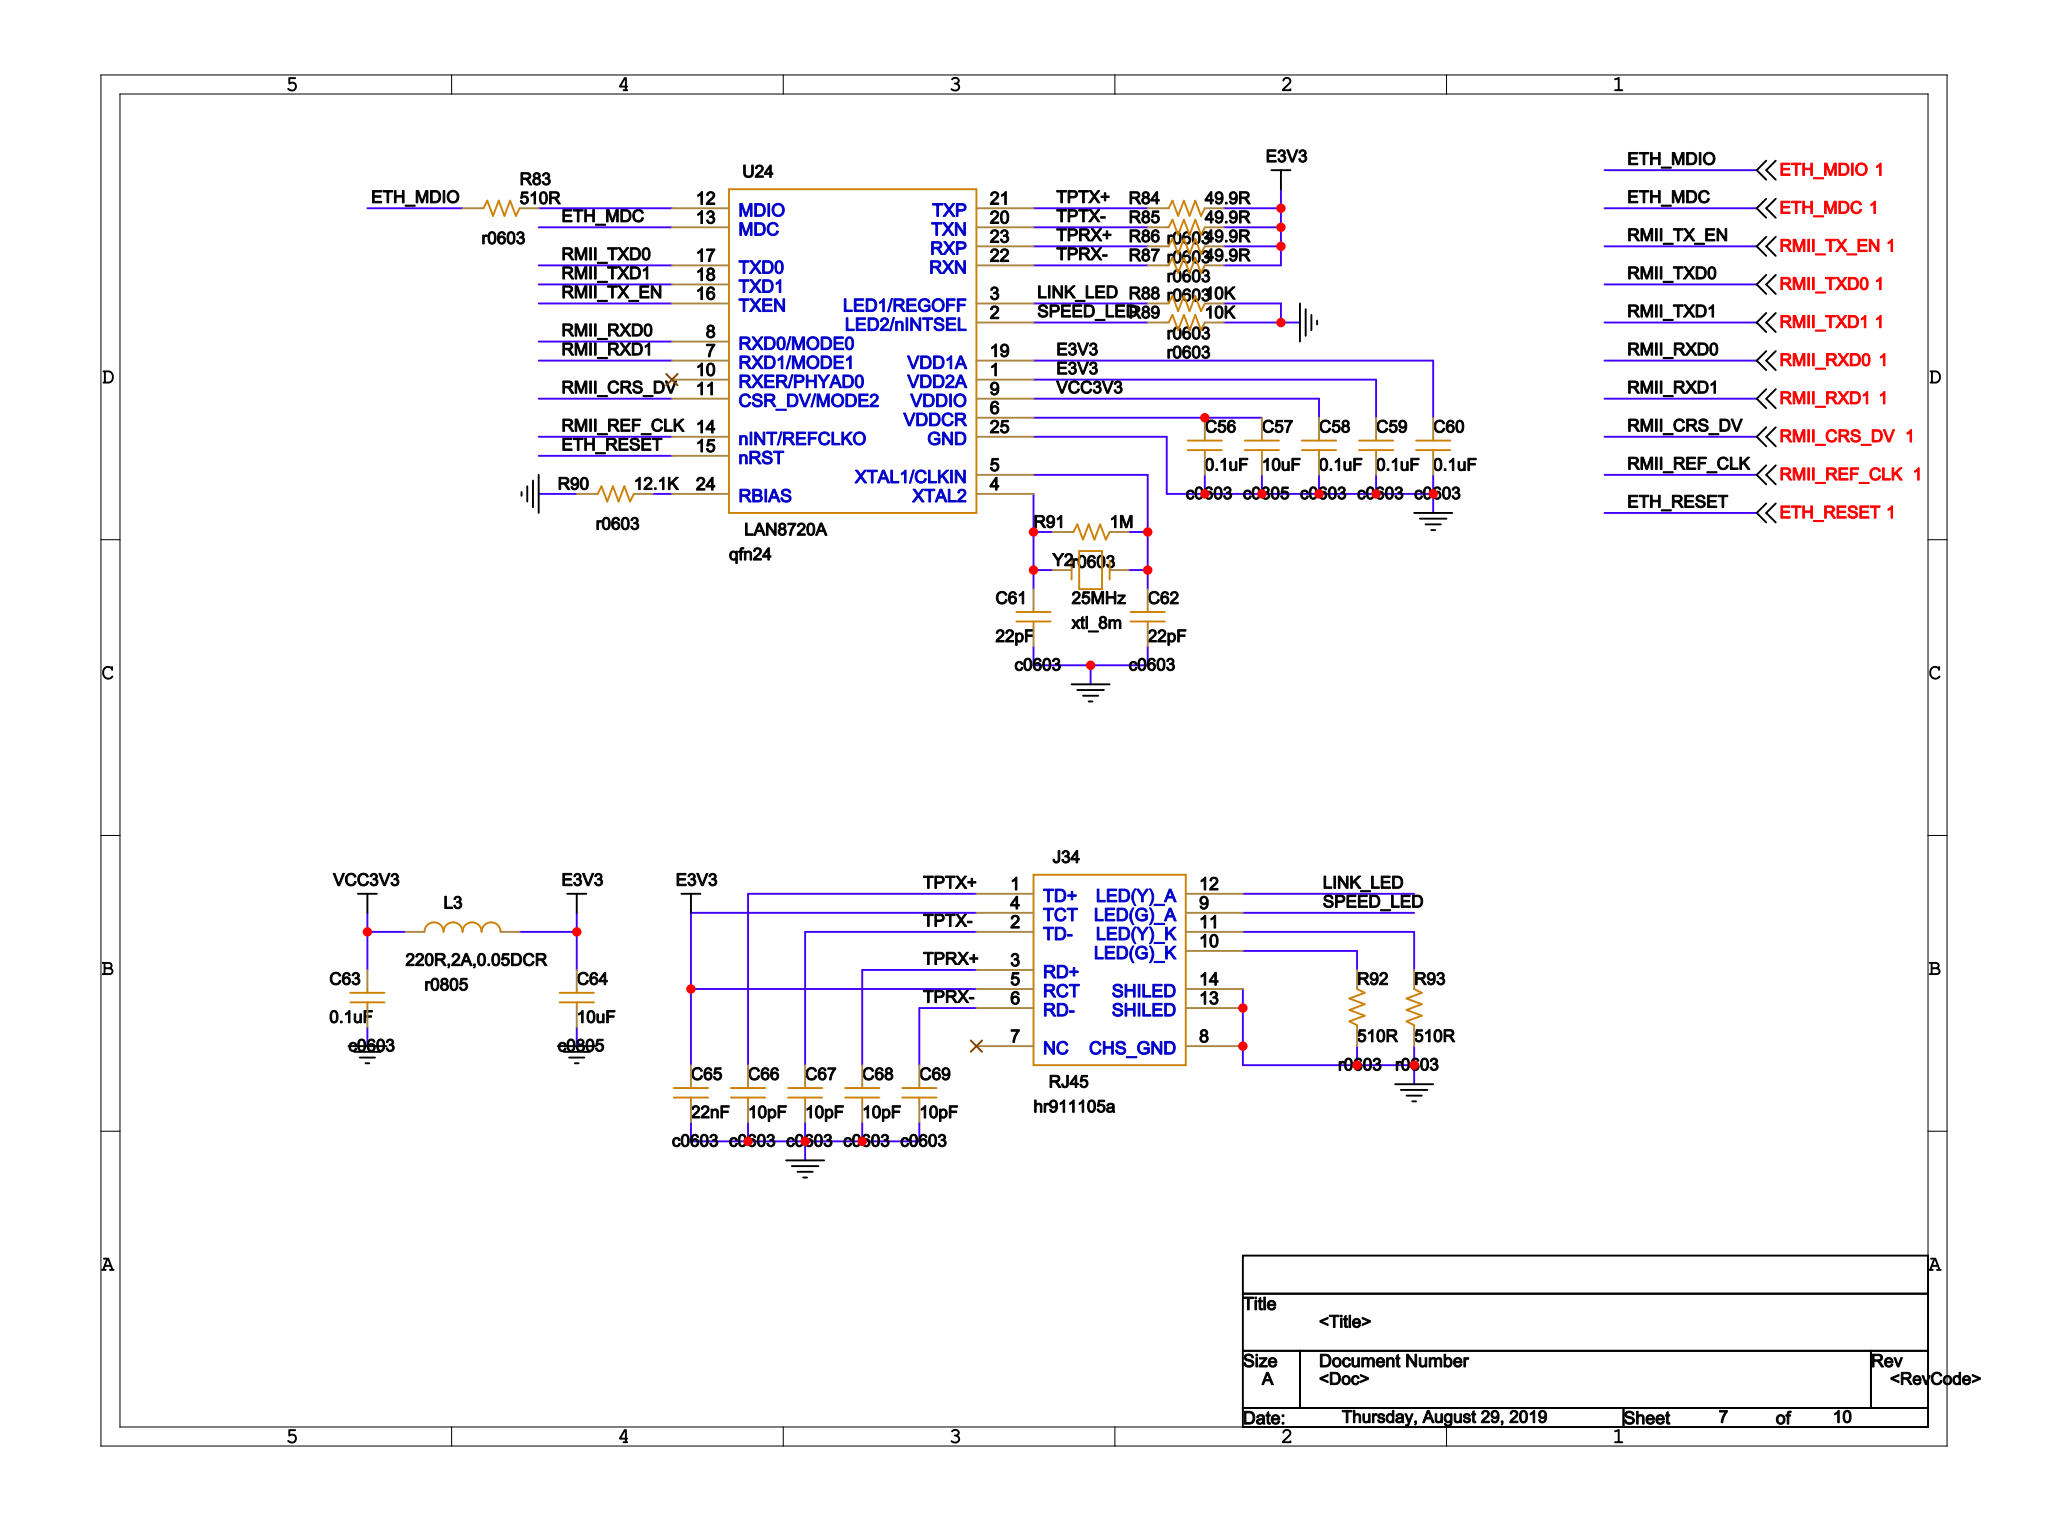Circuit board | Cadence Allegro | 380 parts | 375 nets | one sheet of the schematic
Parts on this sheet (reference | value | footprint):
C56 | 0.1uF | C0603
C57 | 10uF | C0805
C58 | 0.1uF | C0603
C59 | 0.1uF | C0603
C60 | 0.1uF | C0603
C61 | 22pF | C0603
C62 | 22pF | C0603
C63 | 0.1uF | C0603
C64 | 10uF | C0805
C65 | 22nF | C0603
C66 | 10pF | C0603
C67 | 10pF | C0603
C68 | 10pF | C0603
C69 | 10pF | C0603
J34 | RJ45 | HR911105A
L3 | 220R,2A,0.05DCR | R0805
R83 | 510R | R0603
R84 | 49.9R | R0603
R85 | 49.9R | R0603
R86 | 49.9R | R0603
R87 | 49.9R | R0603
R88 | 10K | R0603
R89 | 10K | R0603
R90 | 12.1K | R0603
R91 | 1M | R0603
R93 | 510R | R0603
U24 | LAN8720A | QFN24
Nets of these parts (net: part-pin ...):
GND: C56-2 C57-2 C58-2 C59-2 C60-2 C61-2 C62-2 C63-2 C64-2 C65-2 C66-2 C67-2 C68-2 C69-2 J34-8 J34-13 J34-14 R88-2 R89-2 R90-1 R93-1 U24-25
VCC3V3: C58-1 C63-1 L3-1 U24-9
N1553251: C56-1 C57-1 U24-6
E3V3: C59-1 C60-1 C64-1 C65-1 J34-4 J34-5 L3-2 R84-2 R85-2 R86-2 R87-2 U24-1 U24-19
N1553575: C61-1 R91-1 U24-4
N1553601: C62-1 R91-2 U24-5
TPTX+: C66-1 J34-1 R84-1 U24-21
TPTX-: C67-1 J34-2 R85-1 U24-20
TPRX+: C68-1 J34-3 R86-1 U24-23
TPRX-: C69-1 J34-6 R87-1 U24-22
SPEED_LED: J34-9 R89-1 U24-2
N1555171: J34-10
LINK_LED: J34-12 R88-1 U24-3
N1555158: J34-11 R93-2
ETH_MDIO: R83-1
N1552515: R83-2 U24-12
N1552635: R90-2 U24-24
RMII_REF_CLK: U24-14
RMII_CRS_DV: U24-11
ETH_RESET: U24-15
RMII_TX_EN: U24-16
RMII_TXD0: U24-17
RMII_TXD1: U24-18
ETH_MDC: U24-13
RMII_RXD0: U24-8
RMII_RXD1: U24-7